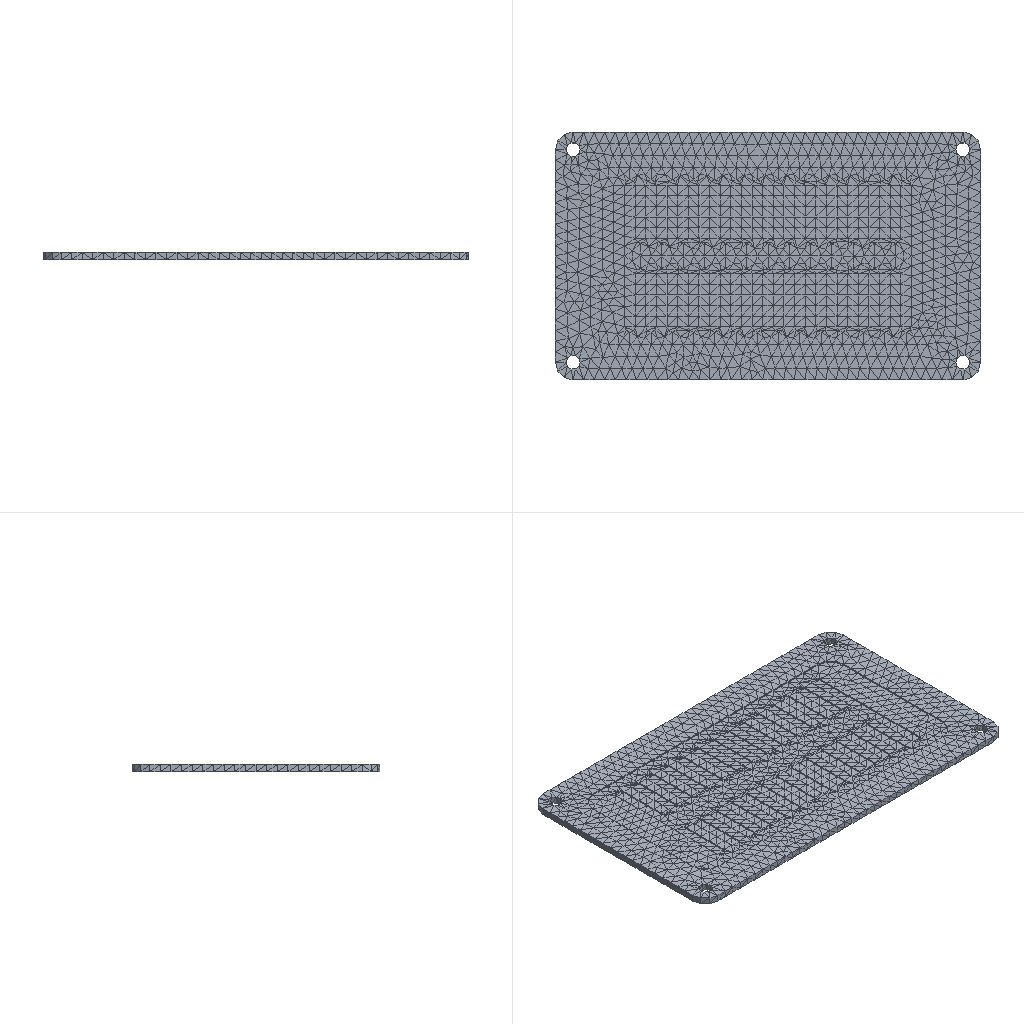Simulation study | ansys workbench
Set-up summary:
category,name,step,type,value,unit,region
solver,ansys_workbench
units,mm-N-s-tonne (MPa),,stated,"/units,MPA"
analysis,LS1,,steady-state thermal
load_step,LS1,LS1,steady-state thermal,nsubst=1; time=1
mesh,nodes,,,17413
mesh,elements,,,10069
element_type,SOLID291,,,8543
element_type,SURF152,,,1526
material,Structural Steel,,E,200000,tonne s^-2 mm^-1
material,Structural Steel,,nu,0.3
material,Structural Steel,,density,7.85e-09,tonne mm^-3
material,Structural Steel,,conductivity,60.5,tonne mm s^-3 C^-1
material,Structural Steel,,specific_heat,4.34e+08,mm^2 s^-2 C^-1
material,Structural Steel,,cte,1.2e-05,C^-1
material,Structural Steel,,permeability,10000
material,Structural Steel,,resistivity,0.00017,ohm mm
load,Define Uniform Initial temperature,model,body load temp,25,,all
load,"Create ""______""",LS1,convection,25000,,SURF152 #2
bc,,LS1,temperature,150 [dofs=TEMP n=2],,node list
named_set,_CM33,,node,4161
named_set,_CM42,,node,6017
Ansys APDL input file, long lists of numbers shortened:
/batch
/config,noeldb,1     ! force off writing results to database
*get,_wallstrt,active,,time,wall
! ANSYS input file written by Workbench version 2022 R1
! File used for geometry attach:
/title,wbnew--___ (B5)
! ****** Begin Custom Load Command Snippet ******
/COM, ACT Extensions:
/COM,     LSDYNA, 2021.1
/COM,
! ****** End   Custom Load Command Snippet ******
*DIM,_wb_ProjectScratch_dir,string,248
_wb_ProjectScratch_dir(1) = ''
*DIM,_wb_SolverFiles_dir,string,248
_wb_SolverFiles_dir(1) = ''
*DIM,_wb_userfiles_dir,string,248
_wb_userfiles_dir(1) = ''
/com,--- Data in consistent NMM units. See Solving Units in the help system for more information.
/units,MPA
/nopr
/wb,file,start              !  signify a WB generated input file
/prep7
! Turn off shape checking because checks already performed inside WB mesher.
! See help system for more information.
SHPP,OFF,,NOWARN
/nolist
etcon,set             ! allow ANSYS to choose best KEYOP's for 180x elements, resets any applicable keyopt to MAPDL defaults
/com,*********** Nodes for the whole assembly ***********
nblock,3,,19154
(1i9,3e20.9e3)
        1     5.000000000E+01    -2.000000000E+01     2.000000000E+00
! (17412 more lines like these left out)
-1
/wb,elem,start            !  set before creation of elements
/com,*********** Elements for Body 1 "___-FreeParts|___" ***********
et,1,291
eblock,19,solid,,8543
(19i9)
        1        1        1        1        0        0        0        0       10        0        1      262     1942      428     2957     4558     5183     4557     4559
! (17085 more lines like these left out)
-1
/wb,elem,end               !  done creating elements
/com,*********** Send User Defined Coordinate System(s) ***********
csys,0
toffst,273.15,  ! Temperature offset from absolute zero
/wb,mat,start              !  starting to send materials
/com,*********** Send Materials ***********
Temperature = 'TEMP' ! Temperature
MP,DENS,1,7.85e-09,	! tonne mm^-3
MP,ALPX,1,1.2e-05,	! C^-1
MP,C,1,434000000,	! mm^2 s^-2 C^-1
MP,KXX,1,60.5,	! tonne mm s^-3 C^-1
MP,RSVX,1,0.00017,	! ohm mm
MP,EX,1,200000,	! tonne s^-2 mm^-1
MP,NUXY,1,0.3,
MP,MURX,1,10000,
/wb,mat,end                !  done sending materials
!************************* Model Summary ********************
!___-FreeParts|___,	结构钢,	matid,	1
!************************* End Model Summary ********************
! get the diagonal of the bounding box. Needed later for other things
*get,_xmin,node,,mnloc,x
*get,_ymin,node,,mnloc,y
*get,_zmin,node,,mnloc,z
*get,_xmax,node,,mxloc,x
*get,_ymax,node,,mxloc,y
*get,_zmax,node,,mxloc,z
_ASMDIAG=(_xmax-_xmin)*(_xmax-_xmin)+(_ymax-_ymin)*(_ymax-_ymin)+(_zmax-_zmin)*(_zmax-_zmin)
_ASMDIAG=SQRT(_ASMDIAG)
/wb,contact,start          !  starting to send contact
/wb,contact,end            !  done creating contacts
/golist
/wb,load,start             !  starting to send loads
/com,*********** Define Temperature Constraint ***********
CMBLOCK,_CM33   ,NODE,     4161
(8i10)
       433       434       435       436       437       438       439       440
! (520 more lines like these left out)
/com,*********** Define Temperature Constraint ***********
CMBLOCK,_CM42   ,NODE,     6017
(8i10)
         1         2         3         4         5         6         7         8
! (752 more lines like these left out)
fcum,add                   ! add nodal forces up (needed in case have loads on the same edge,vertex)
fcum                       ! reset default on fcum command since done sending WB F loads
/com,*********** Create "______" ***********
et,2,152
eblock,10,,,1526
(15i9)
    14406        2        2        2        0     1348     1336     1347     1347    10834    10833     1347    10903
! (1525 more lines like these left out)
-1
esel,s,type,,2
keyop,2,8,2.
keyop,2,13,0
esel,all
/com,***************** Define Uniform Initial temperature ***************
tunif,25.
/gst,on,on
fini
*get,_numnode,node,0,count
*get,_numelem,elem,0,count
*get, _MAXELEMNUM, elem, 0, NUM, MAX
*get, _MAXNODENUM, node, 0, NUM, MAX
*get, _MAXELEMTYPE, etyp, 0, NUM, MAX
*get, _MAXREALCONST, real, 0, NUM, MAX
/go
/wb,load,end               !  done creating loads
/com,--- Number of total nodes = %_numnode%
/com,--- Number of contact elements = 1526
/com,--- Number of spring elements = 0
/com,--- Number of bearing elements = 0
/com,--- Number of solid elements = 8543
/com,--- Number of condensed parts = 0
/com,--- Number of total elements = %_numelem%
*get,_wallbsol,active,,time,wall
/com,****************************************************************************
/com,*************************    SOLUTION       ********************************
/com,****************************************************************************
/solu
antype,0                   ! static analysis
!eqsl,sparse               ! using sparse solver which is default so no eqsl command needed
cntr,print,1               ! print out contact info and also make no initial contact an error
rescontrol,,none                 ! Do not keep any restart files
dmpoption,emat,no             ! Don't combine emat file for DANSYS
dmpoption,esav,no             ! Don't combine esav file for DANSYS
/com,****************************************************
/com,******************* SOLVE FOR LS 1 OF 1 ****************
d,_CM33,temp,150.
d,_CM42,temp,120.
esel,s,type,,2
nsle
sf,all,conv,25000.,150.
nsel,all
esel,all
/nopr
/gopr
autots,on
nsub,1,10,1
time,1.
outres,erase
outres,all,none
outres,nsol,all
outres,rsol,all
outres,eangl,all
outres,veng,all
outres,fflux,all
outres,cont,all
/nopr
esel,s,type,,2
cm,_elmisc,elem
esel,all
/gopr
outres,misc,all,_elmisc
cnvtol,heat,,.001,,1.e-003    ! Program Controlled. Set MINREF equivalent of 1e-6 Watts
! *********** WB SOLVE COMMAND ***********
! check interactive state
*get,ANSINTER_,active,,int
*if,ANSINTER_,ne,0,then
/eof
*endif
solve
/com *************** Write FE CONNECTORS *********
CEWRITE,file,ce,,INTE
/com,****************************************************
/com,*************** FINISHED SOLVE FOR LS 1 *************
*get,_wallasol,active,,time,wall
/post1
xmlo,ENCODING,ISO-8859-1
xmlo,parm
/xml,parm,xml
fini
/gopr
*get,_walldone,active,,time,wall
_preptime=(_wallbsol-_wallstrt)*3600
_solvtime=(_wallasol-_wallbsol)*3600
_posttime=(_walldone-_wallasol)*3600
_totaltim=(_walldone-_wallstrt)*3600
*get,_dlbratio,active,0,solu,dlbr
*get,_combtime,active,0,solu,comb
*get,_ssmode,active,0,solu,ssmm
*get,_ndofs,active,0,solu,ndof
/fclean				!clean distributed files
/com,--- Total number of nodes = %_numnode%
/com,--- Total number of elements = %_numelem%
/com,--- Element load balance ratio = %_dlbratio%
/com,--- Time to combine distributed files = %_combtime%
/com,--- Sparse memory mode = %_ssmode%
/com,--- Number of DOF = %_ndofs%
/wb,file,end               ! done with WB generated input
Results summary:
result,analyses[0].index,,,1
result,analyses[0].system,,,SYS
result,analyses[0].deck,,,deck.dat
result,analyses[0].solve_status,,,completed
result,analyses[0].analysis_type,,,static
result,analyses[0].physics,,,thermal
result,analyses[0].unit_system,,,"NMM: mm, ton, N, s, mV, mA, degC"
result,analyses[0].n_sets,,,1
result,analyses[0].load_steps[0].set,set=1,,1
result,analyses[0].load_steps[0].time_or_freq,set=1,,1
result,analyses[0].load_steps[0].max_temperature,set=1,,150.891
result,analyses[0].load_steps[0].min_temperature,set=1,,118.137